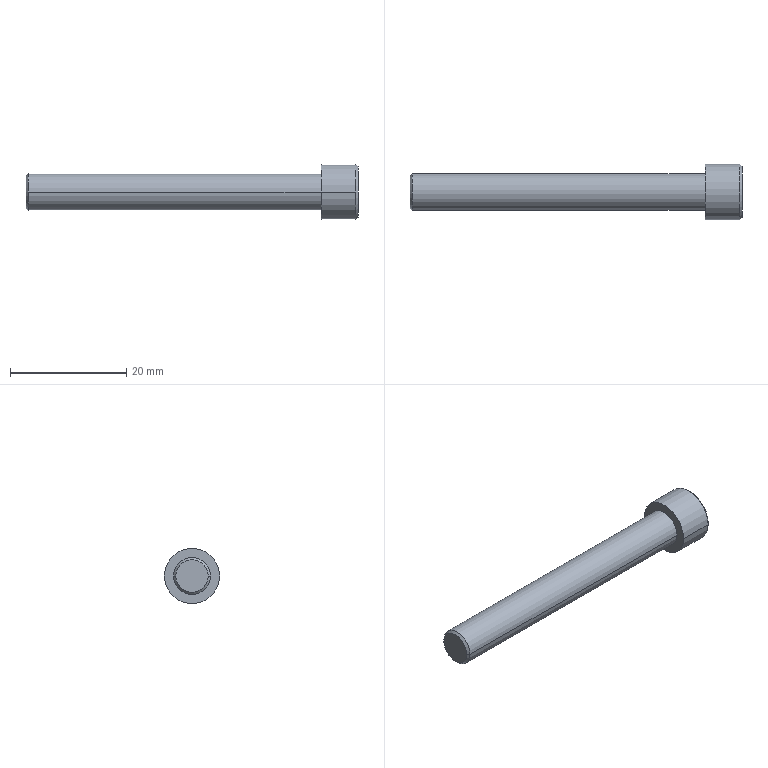Part | STEP file | 4-20.sldasm-Part-46 | 1 solid | 18 faces | box 57.15 x 9.525 x 9.525 mm | volume 2014 mm3 | plane 10 | cone 4 | cylinder 4 | commonest cylinder face diameters 6.35 x2 9.525 x2
STEP:
#1=CARTESIAN_POINT('',(210.776,-426.294,248.05));
#2=VERTEX_POINT('',#1);
#3=CARTESIAN_POINT('',(210.776,-420.706,248.05));
#4=VERTEX_POINT('',#3);
#5=CARTESIAN_POINT('',(210.776,-423.5,248.05));
#6=DIRECTION('',(-1.,0.,0.));
#7=DIRECTION('',(0.,-1.,0.));
#8=AXIS2_PLACEMENT_3D('',#5,#6,#7);
#9=CIRCLE('',#8,2.794);
#10=EDGE_CURVE('',#2,#4,#9,.T.);
#11=ORIENTED_EDGE('',*,*,#10,.F.);
#12=CARTESIAN_POINT('',(211.157,-426.675,248.05));
#13=VERTEX_POINT('',#12);
#14=CARTESIAN_POINT('',(211.157,-426.675,248.05));
#15=DIRECTION('',(0.7071,-0.7071,0.));
#16=VECTOR('',#15,1000.);
#17=LINE('',#14,#16);
#18=EDGE_CURVE('',#2,#13,#17,.T.);
#19=ORIENTED_EDGE('',*,*,#18,.T.);
#20=CARTESIAN_POINT('',(211.157,-420.325,248.05));
#21=VERTEX_POINT('',#20);
#22=CARTESIAN_POINT('',(211.157,-423.5,248.05));
#23=DIRECTION('',(1.,0.,0.));
#24=DIRECTION('',(0.,-1.,0.));
#25=AXIS2_PLACEMENT_3D('',#22,#23,#24);
#26=CIRCLE('',#25,3.175);
#27=EDGE_CURVE('',#21,#13,#26,.T.);
#28=ORIENTED_EDGE('',*,*,#27,.F.);
#29=CARTESIAN_POINT('',(211.157,-420.325,248.05));
#30=DIRECTION('',(0.7071,0.7071,0.));
#31=VECTOR('',#30,1000.);
#32=LINE('',#29,#31);
#33=EDGE_CURVE('',#4,#21,#32,.T.);
#34=ORIENTED_EDGE('',*,*,#33,.F.);
#35=EDGE_LOOP('',(#11,#19,#28,#34));
#36=FACE_OUTER_BOUND('',#35,.T.);
#37=CARTESIAN_POINT('',(211.157,-423.5,248.05));
#38=DIRECTION('',(1.,0.,0.));
#39=DIRECTION('',(0.,1.,0.));
#40=AXIS2_PLACEMENT_3D('',#37,#38,#39);
#41=CONICAL_SURFACE('',#40,3.175,0.7854);
#42=ADVANCED_FACE('',(#36),#41,.T.);
#43=CARTESIAN_POINT('',(267.926,-419.118,248.05));
#44=VERTEX_POINT('',#43);
#45=CARTESIAN_POINT('',(267.926,-427.881,248.05));
#46=VERTEX_POINT('',#45);
#47=CARTESIAN_POINT('',(267.926,-423.5,248.05));
#48=DIRECTION('',(1.,0.,0.));
#49=DIRECTION('',(0.,-1.,0.));
#50=AXIS2_PLACEMENT_3D('',#47,#48,#49);
#51=CIRCLE('',#50,4.381);
#52=EDGE_CURVE('',#44,#46,#51,.T.);
#53=ORIENTED_EDGE('',*,*,#52,.F.);
#54=CARTESIAN_POINT('',(267.545,-418.738,248.05));
#55=VERTEX_POINT('',#54);
#56=CARTESIAN_POINT('',(267.926,-419.118,248.05));
#57=DIRECTION('',(-0.7071,0.7071,0.));
#58=VECTOR('',#57,1000.);
#59=LINE('',#56,#58);
#60=EDGE_CURVE('',#44,#55,#59,.T.);
#61=ORIENTED_EDGE('',*,*,#60,.T.);
#62=CARTESIAN_POINT('',(267.545,-428.262,248.05));
#63=VERTEX_POINT('',#62);
#64=CARTESIAN_POINT('',(267.545,-423.5,248.05));
#65=DIRECTION('',(-1.,0.,0.));
#66=DIRECTION('',(0.,-1.,0.));
#67=AXIS2_PLACEMENT_3D('',#64,#65,#66);
#68=CIRCLE('',#67,4.763);
#69=EDGE_CURVE('',#63,#55,#68,.T.);
#70=ORIENTED_EDGE('',*,*,#69,.F.);
#71=CARTESIAN_POINT('',(267.926,-427.881,248.05));
#72=DIRECTION('',(-0.7071,-0.7071,0.));
#73=VECTOR('',#72,1000.);
#74=LINE('',#71,#73);
#75=EDGE_CURVE('',#46,#63,#74,.T.);
#76=ORIENTED_EDGE('',*,*,#75,.F.);
#77=EDGE_LOOP('',(#53,#61,#70,#76));
#78=FACE_OUTER_BOUND('',#77,.T.);
#79=CARTESIAN_POINT('',(267.926,-423.5,248.05));
#80=DIRECTION('',(-1.,0.,0.));
#81=DIRECTION('',(0.,-1.,0.));
#82=AXIS2_PLACEMENT_3D('',#79,#80,#81);
#83=CONICAL_SURFACE('',#82,4.381,0.7854);
#84=ADVANCED_FACE('',(#78),#83,.T.);
#85=ORIENTED_EDGE('',*,*,#27,.T.);
#86=CARTESIAN_POINT('',(261.576,-426.675,248.05));
#87=VERTEX_POINT('',#86);
#88=CARTESIAN_POINT('',(210.776,-426.675,248.05));
#89=DIRECTION('',(1.,0.,0.));
#90=VECTOR('',#89,1000.);
#91=LINE('',#88,#90);
#92=EDGE_CURVE('',#13,#87,#91,.T.);
#93=ORIENTED_EDGE('',*,*,#92,.T.);
#94=CARTESIAN_POINT('',(261.576,-420.325,248.05));
#95=VERTEX_POINT('',#94);
#96=CARTESIAN_POINT('',(261.576,-423.5,248.05));
#97=DIRECTION('',(1.,0.,0.));
#98=DIRECTION('',(0.,-1.,0.));
#99=AXIS2_PLACEMENT_3D('',#96,#97,#98);
#100=CIRCLE('',#99,3.175);
#101=EDGE_CURVE('',#95,#87,#100,.T.);
#102=ORIENTED_EDGE('',*,*,#101,.F.);
#103=CARTESIAN_POINT('',(210.776,-420.325,248.05));
#104=DIRECTION('',(1.,0.,0.));
#105=VECTOR('',#104,1000.);
#106=LINE('',#103,#105);
#107=EDGE_CURVE('',#21,#95,#106,.T.);
#108=ORIENTED_EDGE('',*,*,#107,.F.);
#109=EDGE_LOOP('',(#85,#93,#102,#108));
#110=FACE_OUTER_BOUND('',#109,.T.);
#111=CARTESIAN_POINT('',(210.776,-423.5,248.05));
#112=DIRECTION('',(1.,0.,0.));
#113=DIRECTION('',(0.,1.,0.));
#114=AXIS2_PLACEMENT_3D('',#111,#112,#113);
#115=CYLINDRICAL_SURFACE('',#114,3.175);
#116=ADVANCED_FACE('',(#110),#115,.T.);
#117=ORIENTED_EDGE('',*,*,#69,.T.);
#118=CARTESIAN_POINT('',(261.576,-418.738,248.05));
#119=VERTEX_POINT('',#118);
#120=CARTESIAN_POINT('',(267.926,-418.738,248.05));
#121=DIRECTION('',(-1.,0.,0.));
#122=VECTOR('',#121,1000.);
#123=LINE('',#120,#122);
#124=EDGE_CURVE('',#55,#119,#123,.T.);
#125=ORIENTED_EDGE('',*,*,#124,.T.);
#126=CARTESIAN_POINT('',(261.576,-428.262,248.05));
#127=VERTEX_POINT('',#126);
#128=CARTESIAN_POINT('',(261.576,-423.5,248.05));
#129=DIRECTION('',(1.,0.,0.));
#130=DIRECTION('',(0.,-1.,0.));
#131=AXIS2_PLACEMENT_3D('',#128,#129,#130);
#132=CIRCLE('',#131,4.763);
#133=EDGE_CURVE('',#119,#127,#132,.T.);
#134=ORIENTED_EDGE('',*,*,#133,.T.);
#135=CARTESIAN_POINT('',(267.926,-428.262,248.05));
#136=DIRECTION('',(-1.,0.,0.));
#137=VECTOR('',#136,1000.);
#138=LINE('',#135,#137);
#139=EDGE_CURVE('',#63,#127,#138,.T.);
#140=ORIENTED_EDGE('',*,*,#139,.F.);
#141=EDGE_LOOP('',(#117,#125,#134,#140));
#142=FACE_OUTER_BOUND('',#141,.T.);
#143=CARTESIAN_POINT('',(267.926,-423.5,248.05));
#144=DIRECTION('',(-1.,0.,0.));
#145=DIRECTION('',(0.,-1.,0.));
#146=AXIS2_PLACEMENT_3D('',#143,#144,#145);
#147=CYLINDRICAL_SURFACE('',#146,4.763);
#148=ADVANCED_FACE('',(#142),#147,.T.);
#149=CARTESIAN_POINT('',(267.926,-423.5,248.05));
#150=DIRECTION('',(1.,0.,0.));
#151=DIRECTION('',(0.,-1.,0.));
#152=AXIS2_PLACEMENT_3D('',#149,#150,#151);
#153=CIRCLE('',#152,4.381);
#154=EDGE_CURVE('',#46,#44,#153,.T.);
#155=ORIENTED_EDGE('',*,*,#154,.T.);
#156=ORIENTED_EDGE('',*,*,#52,.T.);
#157=EDGE_LOOP('',(#155,#156));
#158=FACE_OUTER_BOUND('',#157,.T.);
#159=CARTESIAN_POINT('',(267.926,-422.355,246.066));
#160=VERTEX_POINT('',#159);
#161=CARTESIAN_POINT('',(267.926,-424.645,246.066));
#162=VERTEX_POINT('',#161);
#163=CARTESIAN_POINT('',(267.926,-422.355,246.066));
#164=DIRECTION('',(0.,-1.,0.));
#165=VECTOR('',#164,1000.);
#166=LINE('',#163,#165);
#167=EDGE_CURVE('',#160,#162,#166,.T.);
#168=ORIENTED_EDGE('',*,*,#167,.T.);
#169=CARTESIAN_POINT('',(267.926,-425.791,248.05));
#170=VERTEX_POINT('',#169);
#171=CARTESIAN_POINT('',(267.926,-424.645,246.066));
#172=DIRECTION('',(0.,-0.5,0.866));
#173=VECTOR('',#172,1000.);
#174=LINE('',#171,#173);
#175=EDGE_CURVE('',#162,#170,#174,.T.);
#176=ORIENTED_EDGE('',*,*,#175,.T.);
#177=CARTESIAN_POINT('',(267.926,-424.645,250.034));
#178=VERTEX_POINT('',#177);
#179=CARTESIAN_POINT('',(267.926,-425.791,248.05));
#180=DIRECTION('',(0.,0.5,0.866));
#181=VECTOR('',#180,1000.);
#182=LINE('',#179,#181);
#183=EDGE_CURVE('',#170,#178,#182,.T.);
#184=ORIENTED_EDGE('',*,*,#183,.T.);
#185=CARTESIAN_POINT('',(267.926,-422.355,250.034));
#186=VERTEX_POINT('',#185);
#187=CARTESIAN_POINT('',(267.926,-424.645,250.034));
#188=DIRECTION('',(0.,1.,0.));
#189=VECTOR('',#188,1000.);
#190=LINE('',#187,#189);
#191=EDGE_CURVE('',#178,#186,#190,.T.);
#192=ORIENTED_EDGE('',*,*,#191,.T.);
#193=CARTESIAN_POINT('',(267.926,-421.209,248.05));
#194=VERTEX_POINT('',#193);
#195=CARTESIAN_POINT('',(267.926,-422.355,250.034));
#196=DIRECTION('',(0.,0.5,-0.866));
#197=VECTOR('',#196,1000.);
#198=LINE('',#195,#197);
#199=EDGE_CURVE('',#186,#194,#198,.T.);
#200=ORIENTED_EDGE('',*,*,#199,.T.);
#201=CARTESIAN_POINT('',(267.926,-421.209,248.05));
#202=DIRECTION('',(0.,-0.5,-0.866));
#203=VECTOR('',#202,1000.);
#204=LINE('',#201,#203);
#205=EDGE_CURVE('',#194,#160,#204,.T.);
#206=ORIENTED_EDGE('',*,*,#205,.T.);
#207=EDGE_LOOP('',(#168,#176,#184,#192,#200,#206));
#208=FACE_BOUND('',#207,.T.);
#209=CARTESIAN_POINT('',(267.926,-423.5,248.05));
#210=DIRECTION('',(1.,0.,0.));
#211=DIRECTION('',(0.,1.,0.));
#212=AXIS2_PLACEMENT_3D('',#209,#210,#211);
#213=PLANE('',#212);
#214=ADVANCED_FACE('',(#158,#208),#213,.T.);
#215=ORIENTED_EDGE('',*,*,#124,.F.);
#216=CARTESIAN_POINT('',(267.545,-423.5,248.05));
#217=DIRECTION('',(-1.,0.,0.));
#218=DIRECTION('',(0.,-1.,0.));
#219=AXIS2_PLACEMENT_3D('',#216,#217,#218);
#220=CIRCLE('',#219,4.763);
#221=EDGE_CURVE('',#55,#63,#220,.T.);
#222=ORIENTED_EDGE('',*,*,#221,.T.);
#223=ORIENTED_EDGE('',*,*,#139,.T.);
#224=CARTESIAN_POINT('',(261.576,-423.5,248.05));
#225=DIRECTION('',(1.,0.,0.));
#226=DIRECTION('',(0.,-1.,0.));
#227=AXIS2_PLACEMENT_3D('',#224,#225,#226);
#228=CIRCLE('',#227,4.763);
#229=EDGE_CURVE('',#127,#119,#228,.T.);
#230=ORIENTED_EDGE('',*,*,#229,.T.);
#231=EDGE_LOOP('',(#215,#222,#223,#230));
#232=FACE_OUTER_BOUND('',#231,.T.);
#233=CARTESIAN_POINT('',(267.926,-423.5,248.05));
#234=DIRECTION('',(-1.,0.,0.));
#235=DIRECTION('',(0.,-1.,0.));
#236=AXIS2_PLACEMENT_3D('',#233,#234,#235);
#237=CYLINDRICAL_SURFACE('',#236,4.763);
#238=ADVANCED_FACE('',(#232),#237,.T.);
#239=ORIENTED_EDGE('',*,*,#101,.T.);
#240=CARTESIAN_POINT('',(261.576,-423.5,248.05));
#241=DIRECTION('',(1.,0.,0.));
#242=DIRECTION('',(0.,-1.,0.));
#243=AXIS2_PLACEMENT_3D('',#240,#241,#242);
#244=CIRCLE('',#243,3.175);
#245=EDGE_CURVE('',#87,#95,#244,.T.);
#246=ORIENTED_EDGE('',*,*,#245,.T.);
#247=EDGE_LOOP('',(#239,#246));
#248=FACE_BOUND('',#247,.T.);
#249=ORIENTED_EDGE('',*,*,#229,.F.);
#250=ORIENTED_EDGE('',*,*,#133,.F.);
#251=EDGE_LOOP('',(#249,#250));
#252=FACE_OUTER_BOUND('',#251,.T.);
#253=CARTESIAN_POINT('',(261.576,-423.5,248.05));
#254=DIRECTION('',(1.,0.,0.));
#255=DIRECTION('',(0.,1.,0.));
#256=AXIS2_PLACEMENT_3D('',#253,#254,#255);
#257=PLANE('',#256);
#258=ADVANCED_FACE('',(#248,#252),#257,.F.);
#259=ORIENTED_EDGE('',*,*,#92,.F.);
#260=CARTESIAN_POINT('',(211.157,-423.5,248.05));
#261=DIRECTION('',(1.,0.,0.));
#262=DIRECTION('',(0.,-1.,0.));
#263=AXIS2_PLACEMENT_3D('',#260,#261,#262);
#264=CIRCLE('',#263,3.175);
#265=EDGE_CURVE('',#13,#21,#264,.T.);
#266=ORIENTED_EDGE('',*,*,#265,.T.);
#267=ORIENTED_EDGE('',*,*,#107,.T.);
#268=ORIENTED_EDGE('',*,*,#245,.F.);
#269=EDGE_LOOP('',(#259,#266,#267,#268));
#270=FACE_OUTER_BOUND('',#269,.T.);
#271=CARTESIAN_POINT('',(210.776,-423.5,248.05));
#272=DIRECTION('',(1.,0.,0.));
#273=DIRECTION('',(0.,1.,0.));
#274=AXIS2_PLACEMENT_3D('',#271,#272,#273);
#275=CYLINDRICAL_SURFACE('',#274,3.175);
#276=ADVANCED_FACE('',(#270),#275,.T.);
#277=CARTESIAN_POINT('',(210.776,-423.5,248.05));
#278=DIRECTION('',(-1.,0.,0.));
#279=DIRECTION('',(0.,-1.,0.));
#280=AXIS2_PLACEMENT_3D('',#277,#278,#279);
#281=CIRCLE('',#280,2.794);
#282=EDGE_CURVE('',#4,#2,#281,.T.);
#283=ORIENTED_EDGE('',*,*,#282,.T.);
#284=ORIENTED_EDGE('',*,*,#10,.T.);
#285=EDGE_LOOP('',(#283,#284));
#286=FACE_OUTER_BOUND('',#285,.T.);
#287=CARTESIAN_POINT('',(210.776,-423.5,248.05));
#288=DIRECTION('',(1.,0.,0.));
#289=DIRECTION('',(0.,1.,0.));
#290=AXIS2_PLACEMENT_3D('',#287,#288,#289);
#291=PLANE('',#290);
#292=ADVANCED_FACE('',(#286),#291,.F.);
#293=ORIENTED_EDGE('',*,*,#60,.F.);
#294=ORIENTED_EDGE('',*,*,#154,.F.);
#295=ORIENTED_EDGE('',*,*,#75,.T.);
#296=ORIENTED_EDGE('',*,*,#221,.F.);
#297=EDGE_LOOP('',(#293,#294,#295,#296));
#298=FACE_OUTER_BOUND('',#297,.T.);
#299=CARTESIAN_POINT('',(267.926,-423.5,248.05));
#300=DIRECTION('',(-1.,0.,0.));
#301=DIRECTION('',(0.,-1.,0.));
#302=AXIS2_PLACEMENT_3D('',#299,#300,#301);
#303=CONICAL_SURFACE('',#302,4.381,0.7854);
#304=ADVANCED_FACE('',(#298),#303,.T.);
#305=ORIENTED_EDGE('',*,*,#18,.F.);
#306=ORIENTED_EDGE('',*,*,#282,.F.);
#307=ORIENTED_EDGE('',*,*,#33,.T.);
#308=ORIENTED_EDGE('',*,*,#265,.F.);
#309=EDGE_LOOP('',(#305,#306,#307,#308));
#310=FACE_OUTER_BOUND('',#309,.T.);
#311=CARTESIAN_POINT('',(211.157,-423.5,248.05));
#312=DIRECTION('',(1.,0.,0.));
#313=DIRECTION('',(0.,1.,0.));
#314=AXIS2_PLACEMENT_3D('',#311,#312,#313);
#315=CONICAL_SURFACE('',#314,3.175,0.7854);
#316=ADVANCED_FACE('',(#310),#315,.T.);
#317=ORIENTED_EDGE('',*,*,#175,.F.);
#318=CARTESIAN_POINT('',(264.751,-424.645,246.066));
#319=VERTEX_POINT('',#318);
#320=CARTESIAN_POINT('',(264.751,-424.645,246.066));
#321=DIRECTION('',(1.,0.,0.));
#322=VECTOR('',#321,1000.);
#323=LINE('',#320,#322);
#324=EDGE_CURVE('',#319,#162,#323,.T.);
#325=ORIENTED_EDGE('',*,*,#324,.F.);
#326=CARTESIAN_POINT('',(264.751,-425.791,248.05));
#327=VERTEX_POINT('',#326);
#328=CARTESIAN_POINT('',(264.751,-424.645,246.066));
#329=DIRECTION('',(0.,-0.5,0.866));
#330=VECTOR('',#329,1000.);
#331=LINE('',#328,#330);
#332=EDGE_CURVE('',#319,#327,#331,.T.);
#333=ORIENTED_EDGE('',*,*,#332,.T.);
#334=CARTESIAN_POINT('',(264.751,-425.791,248.05));
#335=DIRECTION('',(1.,0.,0.));
#336=VECTOR('',#335,1000.);
#337=LINE('',#334,#336);
#338=EDGE_CURVE('',#327,#170,#337,.T.);
#339=ORIENTED_EDGE('',*,*,#338,.T.);
#340=EDGE_LOOP('',(#317,#325,#333,#339));
#341=FACE_OUTER_BOUND('',#340,.T.);
#342=CARTESIAN_POINT('',(264.751,-424.645,246.066));
#343=DIRECTION('',(0.,0.866,0.5));
#344=DIRECTION('',(0.,-0.5,0.866));
#345=AXIS2_PLACEMENT_3D('',#342,#343,#344);
#346=PLANE('',#345);
#347=ADVANCED_FACE('',(#341),#346,.T.);
#348=ORIENTED_EDGE('',*,*,#183,.F.);
#349=ORIENTED_EDGE('',*,*,#338,.F.);
#350=CARTESIAN_POINT('',(264.751,-424.645,250.034));
#351=VERTEX_POINT('',#350);
#352=CARTESIAN_POINT('',(264.751,-425.791,248.05));
#353=DIRECTION('',(0.,0.5,0.866));
#354=VECTOR('',#353,1000.);
#355=LINE('',#352,#354);
#356=EDGE_CURVE('',#327,#351,#355,.T.);
#357=ORIENTED_EDGE('',*,*,#356,.T.);
#358=CARTESIAN_POINT('',(264.751,-424.645,250.034));
#359=DIRECTION('',(1.,0.,0.));
#360=VECTOR('',#359,1000.);
#361=LINE('',#358,#360);
#362=EDGE_CURVE('',#351,#178,#361,.T.);
#363=ORIENTED_EDGE('',*,*,#362,.T.);
#364=EDGE_LOOP('',(#348,#349,#357,#363));
#365=FACE_OUTER_BOUND('',#364,.T.);
#366=CARTESIAN_POINT('',(264.751,-425.791,248.05));
#367=DIRECTION('',(0.,0.866,-0.5));
#368=DIRECTION('',(0.,0.5,0.866));
#369=AXIS2_PLACEMENT_3D('',#366,#367,#368);
#370=PLANE('',#369);
#371=ADVANCED_FACE('',(#365),#370,.T.);
#372=ORIENTED_EDGE('',*,*,#191,.F.);
#373=ORIENTED_EDGE('',*,*,#362,.F.);
#374=CARTESIAN_POINT('',(264.751,-422.355,250.034));
#375=VERTEX_POINT('',#374);
#376=CARTESIAN_POINT('',(264.751,-424.645,250.034));
#377=DIRECTION('',(0.,1.,0.));
#378=VECTOR('',#377,1000.);
#379=LINE('',#376,#378);
#380=EDGE_CURVE('',#351,#375,#379,.T.);
#381=ORIENTED_EDGE('',*,*,#380,.T.);
#382=CARTESIAN_POINT('',(264.751,-422.355,250.034));
#383=DIRECTION('',(1.,0.,0.));
#384=VECTOR('',#383,1000.);
#385=LINE('',#382,#384);
#386=EDGE_CURVE('',#375,#186,#385,.T.);
#387=ORIENTED_EDGE('',*,*,#386,.T.);
#388=EDGE_LOOP('',(#372,#373,#381,#387));
#389=FACE_OUTER_BOUND('',#388,.T.);
#390=CARTESIAN_POINT('',(264.751,-424.645,250.034));
#391=DIRECTION('',(0.,0.,-1.));
#392=DIRECTION('',(-1.,0.,0.));
#393=AXIS2_PLACEMENT_3D('',#390,#391,#392);
#394=PLANE('',#393);
#395=ADVANCED_FACE('',(#389),#394,.T.);
#396=ORIENTED_EDGE('',*,*,#199,.F.);
#397=ORIENTED_EDGE('',*,*,#386,.F.);
#398=CARTESIAN_POINT('',(264.751,-421.209,248.05));
#399=VERTEX_POINT('',#398);
#400=CARTESIAN_POINT('',(264.751,-422.355,250.034));
#401=DIRECTION('',(0.,0.5,-0.866));
#402=VECTOR('',#401,1000.);
#403=LINE('',#400,#402);
#404=EDGE_CURVE('',#375,#399,#403,.T.);
#405=ORIENTED_EDGE('',*,*,#404,.T.);
#406=CARTESIAN_POINT('',(264.751,-421.209,248.05));
#407=DIRECTION('',(1.,0.,0.));
#408=VECTOR('',#407,1000.);
#409=LINE('',#406,#408);
#410=EDGE_CURVE('',#399,#194,#409,.T.);
#411=ORIENTED_EDGE('',*,*,#410,.T.);
#412=EDGE_LOOP('',(#396,#397,#405,#411));
#413=FACE_OUTER_BOUND('',#412,.T.);
#414=CARTESIAN_POINT('',(264.751,-422.355,250.034));
#415=DIRECTION('',(0.,-0.866,-0.5));
#416=DIRECTION('',(0.,0.5,-0.866));
#417=AXIS2_PLACEMENT_3D('',#414,#415,#416);
#418=PLANE('',#417);
#419=ADVANCED_FACE('',(#413),#418,.T.);
#420=ORIENTED_EDGE('',*,*,#205,.F.);
#421=ORIENTED_EDGE('',*,*,#410,.F.);
#422=CARTESIAN_POINT('',(264.751,-422.355,246.066));
#423=VERTEX_POINT('',#422);
#424=CARTESIAN_POINT('',(264.751,-421.209,248.05));
#425=DIRECTION('',(0.,-0.5,-0.866));
#426=VECTOR('',#425,1000.);
#427=LINE('',#424,#426);
#428=EDGE_CURVE('',#399,#423,#427,.T.);
#429=ORIENTED_EDGE('',*,*,#428,.T.);
#430=CARTESIAN_POINT('',(264.751,-422.355,246.066));
#431=DIRECTION('',(1.,0.,0.));
#432=VECTOR('',#431,1000.);
#433=LINE('',#430,#432);
#434=EDGE_CURVE('',#423,#160,#433,.T.);
#435=ORIENTED_EDGE('',*,*,#434,.T.);
#436=EDGE_LOOP('',(#420,#421,#429,#435));
#437=FACE_OUTER_BOUND('',#436,.T.);
#438=CARTESIAN_POINT('',(264.751,-421.209,248.05));
#439=DIRECTION('',(0.,-0.866,0.5));
#440=DIRECTION('',(0.,-0.5,-0.866));
#441=AXIS2_PLACEMENT_3D('',#438,#439,#440);
#442=PLANE('',#441);
#443=ADVANCED_FACE('',(#437),#442,.T.);
#444=ORIENTED_EDGE('',*,*,#167,.F.);
#445=ORIENTED_EDGE('',*,*,#434,.F.);
#446=CARTESIAN_POINT('',(264.751,-422.355,246.066));
#447=DIRECTION('',(0.,-1.,0.));
#448=VECTOR('',#447,1000.);
#449=LINE('',#446,#448);
#450=EDGE_CURVE('',#423,#319,#449,.T.);
#451=ORIENTED_EDGE('',*,*,#450,.T.);
#452=ORIENTED_EDGE('',*,*,#324,.T.);
#453=EDGE_LOOP('',(#444,#445,#451,#452));
#454=FACE_OUTER_BOUND('',#453,.T.);
#455=CARTESIAN_POINT('',(264.751,-422.355,246.066));
#456=DIRECTION('',(0.,0.,1.));
#457=DIRECTION('',(1.,0.,0.));
#458=AXIS2_PLACEMENT_3D('',#455,#456,#457);
#459=PLANE('',#458);
#460=ADVANCED_FACE('',(#454),#459,.T.);
#461=ORIENTED_EDGE('',*,*,#332,.F.);
#462=ORIENTED_EDGE('',*,*,#450,.F.);
#463=ORIENTED_EDGE('',*,*,#428,.F.);
#464=ORIENTED_EDGE('',*,*,#404,.F.);
#465=ORIENTED_EDGE('',*,*,#380,.F.);
#466=ORIENTED_EDGE('',*,*,#356,.F.);
#467=EDGE_LOOP('',(#461,#462,#463,#464,#465,#466));
#468=FACE_OUTER_BOUND('',#467,.T.);
#469=CARTESIAN_POINT('',(264.751,-425.791,248.05));
#470=DIRECTION('',(-1.,0.,0.));
#471=DIRECTION('',(0.,-1.,0.));
#472=AXIS2_PLACEMENT_3D('',#469,#470,#471);
#473=PLANE('',#472);
#474=ADVANCED_FACE('',(#468),#473,.F.);
#475=CLOSED_SHELL('',(#42,#84,#116,#148,#214,#238,#258,#276,#292,#304,#316,#347,#371,#395,#419,#443,#460,#474));
#476=MANIFOLD_SOLID_BREP('',#475);
#477=CARTESIAN_POINT('',(0.,0.,0.));
#478=DIRECTION('',(0.,0.,1.));
#479=DIRECTION('',(1.,0.,0.));
#480=AXIS2_PLACEMENT_3D('',#477,#478,#479);
#481=(LENGTH_UNIT()NAMED_UNIT(*)SI_UNIT(.MILLI.,.METRE.));
#482=UNCERTAINTY_MEASURE_WITH_UNIT(LENGTH_MEASURE(0.00001),#481,'','');
#483=(NAMED_UNIT(*)PLANE_ANGLE_UNIT()SI_UNIT($,.RADIAN.));
#484=(NAMED_UNIT(*)SI_UNIT($,.STERADIAN.)SOLID_ANGLE_UNIT());
#485=(GEOMETRIC_REPRESENTATION_CONTEXT(3)GLOBAL_UNCERTAINTY_ASSIGNED_CONTEXT((#482))GLOBAL_UNIT_ASSIGNED_CONTEXT((#481,#483,#484))REPRESENTATION_CONTEXT('',''));
#486=ADVANCED_BREP_SHAPE_REPRESENTATION('',(#476,#480),#485);